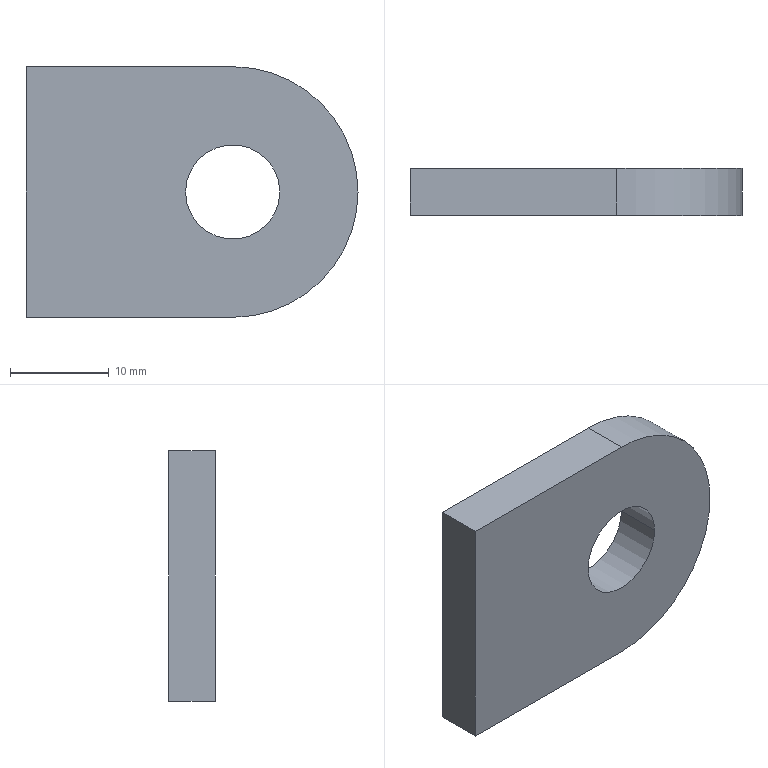Part | NX | features BREP 1 | 1 solid | 8 faces | box 33.655 x 4.763 x 25.4 mm | volume 3400 mm3 | plane 5 | cylinder 3 | commonest cylinder face diameters 9.55 x2 25.4 x1
STEP:
#1=CARTESIAN_POINT('',(0.,0.,12.7));
#2=VERTEX_POINT('',#1);
#3=CARTESIAN_POINT('',(20.955,0.,12.7));
#4=VERTEX_POINT('',#3);
#5=CARTESIAN_POINT('',(0.,0.,12.7));
#6=DIRECTION('',(1.,0.,0.));
#7=VECTOR('',#6,1000.);
#8=LINE('',#5,#7);
#9=EDGE_CURVE('',#2,#4,#8,.T.);
#10=ORIENTED_EDGE('',*,*,#9,.T.);
#11=CARTESIAN_POINT('',(20.955,0.,-12.7));
#12=VERTEX_POINT('',#11);
#13=CARTESIAN_POINT('',(20.955,0.,0.));
#14=DIRECTION('',(0.,1.,0.));
#15=DIRECTION('',(0.,0.,1.));
#16=AXIS2_PLACEMENT_3D('',#13,#14,#15);
#17=CIRCLE('',#16,12.7);
#18=EDGE_CURVE('',#4,#12,#17,.T.);
#19=ORIENTED_EDGE('',*,*,#18,.T.);
#20=CARTESIAN_POINT('',(0.,0.,-12.7));
#21=VERTEX_POINT('',#20);
#22=CARTESIAN_POINT('',(20.955,0.,-12.7));
#23=DIRECTION('',(-1.,0.,0.));
#24=VECTOR('',#23,1000.);
#25=LINE('',#22,#24);
#26=EDGE_CURVE('',#12,#21,#25,.T.);
#27=ORIENTED_EDGE('',*,*,#26,.T.);
#28=CARTESIAN_POINT('',(0.,0.,-12.7));
#29=DIRECTION('',(0.,0.,1.));
#30=VECTOR('',#29,1000.);
#31=LINE('',#28,#30);
#32=EDGE_CURVE('',#21,#2,#31,.T.);
#33=ORIENTED_EDGE('',*,*,#32,.T.);
#34=EDGE_LOOP('',(#10,#19,#27,#33));
#35=FACE_BOUND('',#34,.T.);
#36=CARTESIAN_POINT('',(25.73,0.,0.));
#37=VERTEX_POINT('',#36);
#38=CARTESIAN_POINT('',(16.18,0.,0.));
#39=VERTEX_POINT('',#38);
#40=CARTESIAN_POINT('',(20.955,0.,0.));
#41=DIRECTION('',(0.,1.,0.));
#42=DIRECTION('',(1.,0.,0.));
#43=AXIS2_PLACEMENT_3D('',#40,#41,#42);
#44=CIRCLE('',#43,4.775);
#45=EDGE_CURVE('',#37,#39,#44,.T.);
#46=ORIENTED_EDGE('',*,*,#45,.F.);
#47=CARTESIAN_POINT('',(20.955,0.,0.));
#48=DIRECTION('',(0.,1.,0.));
#49=DIRECTION('',(-1.,0.,0.));
#50=AXIS2_PLACEMENT_3D('',#47,#48,#49);
#51=CIRCLE('',#50,4.775);
#52=EDGE_CURVE('',#39,#37,#51,.T.);
#53=ORIENTED_EDGE('',*,*,#52,.F.);
#54=EDGE_LOOP('',(#46,#53));
#55=FACE_BOUND('',#54,.T.);
#56=CARTESIAN_POINT('',(0.,0.,0.));
#57=DIRECTION('',(0.,1.,0.));
#58=DIRECTION('',(1.,0.,0.));
#59=AXIS2_PLACEMENT_3D('',#56,#57,#58);
#60=PLANE('',#59);
#61=ADVANCED_FACE('',(#35,#55),#60,.T.);
#62=CARTESIAN_POINT('',(0.,-4.763,-12.7));
#63=VERTEX_POINT('',#62);
#64=CARTESIAN_POINT('',(0.,0.,-12.7));
#65=DIRECTION('',(0.,-1.,0.));
#66=VECTOR('',#65,1000.);
#67=LINE('',#64,#66);
#68=EDGE_CURVE('',#21,#63,#67,.T.);
#69=ORIENTED_EDGE('',*,*,#68,.T.);
#70=CARTESIAN_POINT('',(0.,-4.763,12.7));
#71=VERTEX_POINT('',#70);
#72=CARTESIAN_POINT('',(0.,-4.763,-12.7));
#73=DIRECTION('',(0.,0.,1.));
#74=VECTOR('',#73,1000.);
#75=LINE('',#72,#74);
#76=EDGE_CURVE('',#63,#71,#75,.T.);
#77=ORIENTED_EDGE('',*,*,#76,.T.);
#78=CARTESIAN_POINT('',(0.,0.,12.7));
#79=DIRECTION('',(0.,-1.,0.));
#80=VECTOR('',#79,1000.);
#81=LINE('',#78,#80);
#82=EDGE_CURVE('',#2,#71,#81,.T.);
#83=ORIENTED_EDGE('',*,*,#82,.F.);
#84=ORIENTED_EDGE('',*,*,#32,.F.);
#85=EDGE_LOOP('',(#69,#77,#83,#84));
#86=FACE_BOUND('',#85,.T.);
#87=CARTESIAN_POINT('',(0.,-2.381,0.));
#88=DIRECTION('',(-1.,0.,0.));
#89=DIRECTION('',(0.,0.,1.));
#90=AXIS2_PLACEMENT_3D('',#87,#88,#89);
#91=PLANE('',#90);
#92=ADVANCED_FACE('',(#86),#91,.T.);
#93=ORIENTED_EDGE('',*,*,#82,.T.);
#94=CARTESIAN_POINT('',(20.955,-4.763,12.7));
#95=VERTEX_POINT('',#94);
#96=CARTESIAN_POINT('',(0.,-4.763,12.7));
#97=DIRECTION('',(1.,0.,0.));
#98=VECTOR('',#97,1000.);
#99=LINE('',#96,#98);
#100=EDGE_CURVE('',#71,#95,#99,.T.);
#101=ORIENTED_EDGE('',*,*,#100,.T.);
#102=CARTESIAN_POINT('',(20.955,0.,12.7));
#103=DIRECTION('',(0.,-1.,0.));
#104=VECTOR('',#103,1000.);
#105=LINE('',#102,#104);
#106=EDGE_CURVE('',#4,#95,#105,.T.);
#107=ORIENTED_EDGE('',*,*,#106,.F.);
#108=ORIENTED_EDGE('',*,*,#9,.F.);
#109=EDGE_LOOP('',(#93,#101,#107,#108));
#110=FACE_BOUND('',#109,.T.);
#111=CARTESIAN_POINT('',(10.477,-2.381,12.7));
#112=DIRECTION('',(0.,0.,1.));
#113=DIRECTION('',(1.,0.,0.));
#114=AXIS2_PLACEMENT_3D('',#111,#112,#113);
#115=PLANE('',#114);
#116=ADVANCED_FACE('',(#110),#115,.T.);
#117=ORIENTED_EDGE('',*,*,#106,.T.);
#118=CARTESIAN_POINT('',(20.955,-4.763,-12.7));
#119=VERTEX_POINT('',#118);
#120=CARTESIAN_POINT('',(20.955,-4.763,0.));
#121=DIRECTION('',(0.,1.,0.));
#122=DIRECTION('',(0.,0.,1.));
#123=AXIS2_PLACEMENT_3D('',#120,#121,#122);
#124=CIRCLE('',#123,12.7);
#125=EDGE_CURVE('',#95,#119,#124,.T.);
#126=ORIENTED_EDGE('',*,*,#125,.T.);
#127=CARTESIAN_POINT('',(20.955,0.,-12.7));
#128=DIRECTION('',(0.,-1.,0.));
#129=VECTOR('',#128,1000.);
#130=LINE('',#127,#129);
#131=EDGE_CURVE('',#12,#119,#130,.T.);
#132=ORIENTED_EDGE('',*,*,#131,.F.);
#133=ORIENTED_EDGE('',*,*,#18,.F.);
#134=EDGE_LOOP('',(#117,#126,#132,#133));
#135=FACE_BOUND('',#134,.T.);
#136=CARTESIAN_POINT('',(20.955,-2.381,0.));
#137=DIRECTION('',(0.,1.,0.));
#138=DIRECTION('',(0.,0.,1.));
#139=AXIS2_PLACEMENT_3D('',#136,#137,#138);
#140=CYLINDRICAL_SURFACE('',#139,12.7);
#141=ADVANCED_FACE('',(#135),#140,.T.);
#142=ORIENTED_EDGE('',*,*,#131,.T.);
#143=CARTESIAN_POINT('',(20.955,-4.763,-12.7));
#144=DIRECTION('',(-1.,0.,0.));
#145=VECTOR('',#144,1000.);
#146=LINE('',#143,#145);
#147=EDGE_CURVE('',#119,#63,#146,.T.);
#148=ORIENTED_EDGE('',*,*,#147,.T.);
#149=ORIENTED_EDGE('',*,*,#68,.F.);
#150=ORIENTED_EDGE('',*,*,#26,.F.);
#151=EDGE_LOOP('',(#142,#148,#149,#150));
#152=FACE_BOUND('',#151,.T.);
#153=CARTESIAN_POINT('',(10.477,-2.381,-12.7));
#154=DIRECTION('',(0.,0.,-1.));
#155=DIRECTION('',(0.,-1.,0.));
#156=AXIS2_PLACEMENT_3D('',#153,#154,#155);
#157=PLANE('',#156);
#158=ADVANCED_FACE('',(#152),#157,.T.);
#159=ORIENTED_EDGE('',*,*,#147,.F.);
#160=ORIENTED_EDGE('',*,*,#125,.F.);
#161=ORIENTED_EDGE('',*,*,#100,.F.);
#162=ORIENTED_EDGE('',*,*,#76,.F.);
#163=EDGE_LOOP('',(#159,#160,#161,#162));
#164=FACE_BOUND('',#163,.T.);
#165=CARTESIAN_POINT('',(25.73,-4.763,0.));
#166=VERTEX_POINT('',#165);
#167=CARTESIAN_POINT('',(16.18,-4.763,0.));
#168=VERTEX_POINT('',#167);
#169=CARTESIAN_POINT('',(20.955,-4.763,0.));
#170=DIRECTION('',(0.,1.,0.));
#171=DIRECTION('',(1.,0.,0.));
#172=AXIS2_PLACEMENT_3D('',#169,#170,#171);
#173=CIRCLE('',#172,4.775);
#174=EDGE_CURVE('',#166,#168,#173,.T.);
#175=ORIENTED_EDGE('',*,*,#174,.T.);
#176=CARTESIAN_POINT('',(20.955,-4.763,0.));
#177=DIRECTION('',(0.,1.,0.));
#178=DIRECTION('',(-1.,0.,0.));
#179=AXIS2_PLACEMENT_3D('',#176,#177,#178);
#180=CIRCLE('',#179,4.775);
#181=EDGE_CURVE('',#168,#166,#180,.T.);
#182=ORIENTED_EDGE('',*,*,#181,.T.);
#183=EDGE_LOOP('',(#175,#182));
#184=FACE_BOUND('',#183,.T.);
#185=CARTESIAN_POINT('',(0.,-4.763,0.));
#186=DIRECTION('',(0.,1.,0.));
#187=DIRECTION('',(1.,0.,0.));
#188=AXIS2_PLACEMENT_3D('',#185,#186,#187);
#189=PLANE('',#188);
#190=ADVANCED_FACE('',(#164,#184),#189,.F.);
#191=CARTESIAN_POINT('',(25.73,0.,0.));
#192=DIRECTION('',(0.,-1.,0.));
#193=VECTOR('',#192,1000.);
#194=LINE('',#191,#193);
#195=EDGE_CURVE('',#166,#37,#194,.F.);
#196=ORIENTED_EDGE('',*,*,#195,.F.);
#197=ORIENTED_EDGE('',*,*,#181,.F.);
#198=CARTESIAN_POINT('',(16.18,0.,0.));
#199=DIRECTION('',(0.,-1.,0.));
#200=VECTOR('',#199,1000.);
#201=LINE('',#198,#200);
#202=EDGE_CURVE('',#168,#39,#201,.F.);
#203=ORIENTED_EDGE('',*,*,#202,.T.);
#204=ORIENTED_EDGE('',*,*,#52,.T.);
#205=EDGE_LOOP('',(#196,#197,#203,#204));
#206=FACE_BOUND('',#205,.T.);
#207=CARTESIAN_POINT('',(20.955,-2.381,0.));
#208=DIRECTION('',(0.,1.,0.));
#209=DIRECTION('',(-1.,0.,0.));
#210=AXIS2_PLACEMENT_3D('',#207,#208,#209);
#211=CYLINDRICAL_SURFACE('',#210,4.775);
#212=ADVANCED_FACE('',(#206),#211,.F.);
#213=ORIENTED_EDGE('',*,*,#202,.F.);
#214=ORIENTED_EDGE('',*,*,#174,.F.);
#215=ORIENTED_EDGE('',*,*,#195,.T.);
#216=ORIENTED_EDGE('',*,*,#45,.T.);
#217=EDGE_LOOP('',(#213,#214,#215,#216));
#218=FACE_BOUND('',#217,.T.);
#219=CARTESIAN_POINT('',(20.955,-2.381,0.));
#220=DIRECTION('',(0.,1.,0.));
#221=DIRECTION('',(1.,0.,0.));
#222=AXIS2_PLACEMENT_3D('',#219,#220,#221);
#223=CYLINDRICAL_SURFACE('',#222,4.775);
#224=ADVANCED_FACE('',(#218),#223,.F.);
#225=CLOSED_SHELL('',(#61,#92,#116,#141,#158,#190,#212,#224));
#226=MANIFOLD_SOLID_BREP('',#225);
#227=(LENGTH_UNIT()NAMED_UNIT(*)SI_UNIT(.MILLI.,.METRE.));
#228=UNCERTAINTY_MEASURE_WITH_UNIT(LENGTH_MEASURE(0.00001),#227,'','');
#229=(NAMED_UNIT(*)PLANE_ANGLE_UNIT()SI_UNIT($,.RADIAN.));
#230=(NAMED_UNIT(*)SI_UNIT($,.STERADIAN.)SOLID_ANGLE_UNIT());
#231=(GEOMETRIC_REPRESENTATION_CONTEXT(3)GLOBAL_UNCERTAINTY_ASSIGNED_CONTEXT((#228))GLOBAL_UNIT_ASSIGNED_CONTEXT((#227,#229,#230))REPRESENTATION_CONTEXT('',''));
#232=ADVANCED_BREP_SHAPE_REPRESENTATION('',(#226),#231);